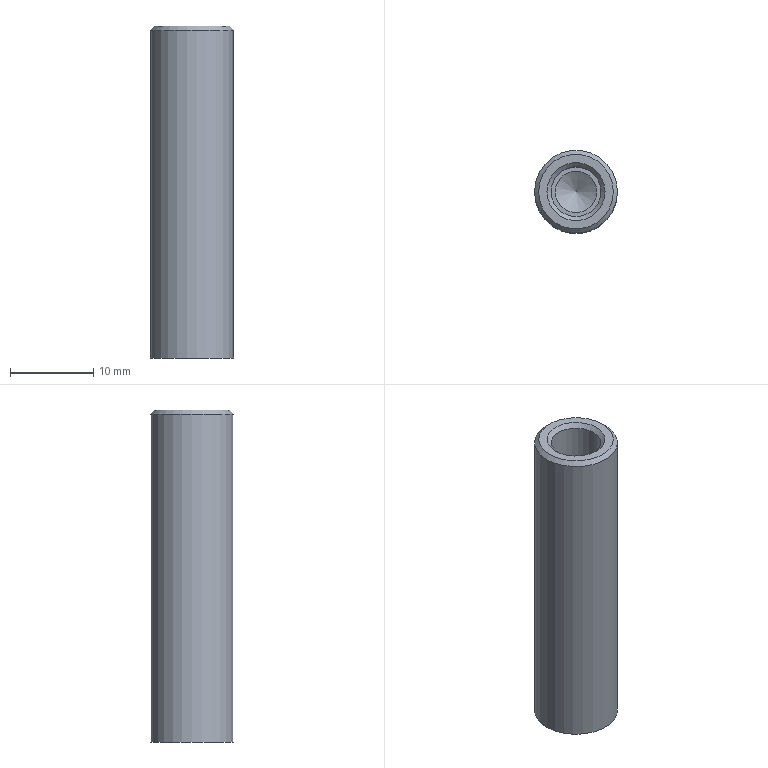Part | STEP file | solid 80 | 1 solid | 9 faces | box 10 x 10 x 40 mm | volume 2747 mm3 | plane 3 | cylinder 3 | cone 3 | commonest cylinder face diameters 5 x1 6 x1 10 x1